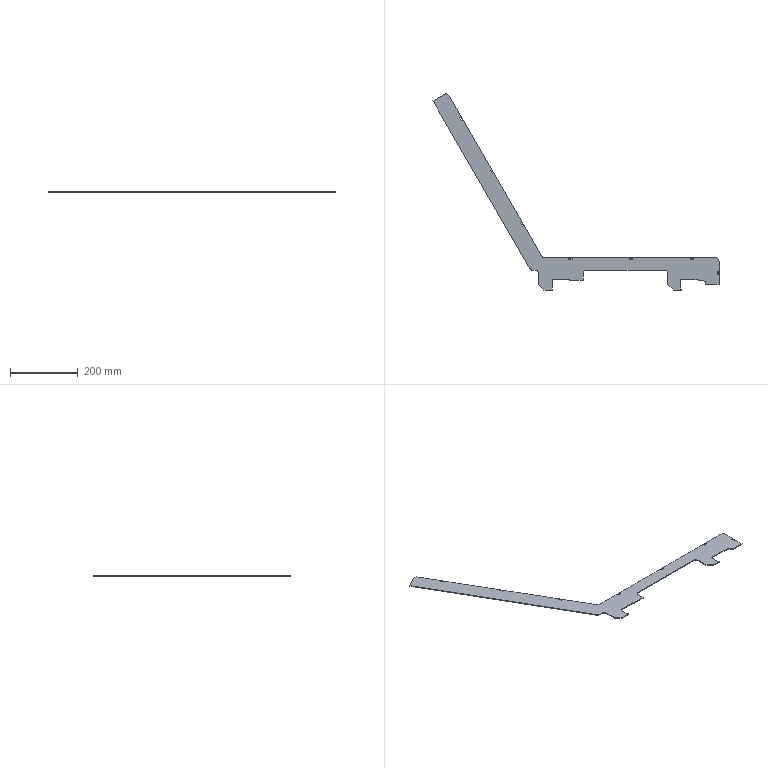Part | STEP file | zq002-1 | 1 solid | 65 faces | box 845.991 x 579.972 x 2 mm | volume 116517 mm3 | plane 58 | cylinder 7 | commonest cylinder face diameters 20 x7